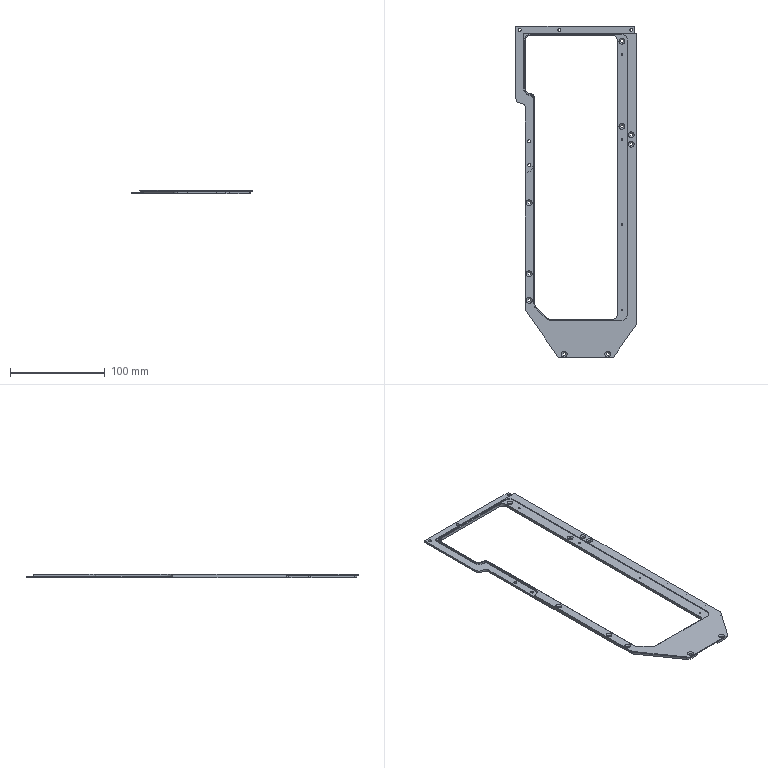NC program | NX | posted with a generic post | part box 127 x 351 x 4 mm
Whole program:
N10 G17 G21 G94 G90
(DRILL_HOLES , TOOL : CHAMFER_D8-90DEG)
N12 T01 M6
N14 G53
N16 G17 G0 G90 X153.952 Y-40.61 S2500 M3
N18 G43 Z20. H1
N20 G94 G82 G98 Z-2.6 F250. P200 R3.
N22 X103.952 Y-30.61
N24 X48.952
N26 X-6.048
N28 X-61.048
N30 X-111.048
N32 X-101. Y3.5
N34 X-111.048 Y28.911
N36 X-61.048
N38 X-6.048
N40 X48.952
N42 X103.952
N44 X119. Y3.5
N46 X153.952 Y28.911
N48 G80
N50 G0 X153.952 Y28.911 Z20.
(DRILL_HOLES_1_COPY_1 , TOOL : CHAMFER_D8-90DEG)
N52 X-168. Y33.5
N54 G82 Z-1.6 F250. P200 R3.
N56 Y-12.5
N58 G80
N60 G0 X-168. Y-12.5 Z20.
N62 M5
(DRILL_HOLES_COPY , TOOL : DRILL_D5.3-62-92)
N64 T02 M6
N66 G53
N68 G17 G0 G90 X153.952 Y-40.61 S3000 M3
N70 G43 Z20. H2
N72 G94 G82 G98 Z-6.5 F200. P200 R3.
N74 X103.952 Y-30.61
N76 X48.952
N78 X-6.048
N80 X-61.048
N82 X-111.048
N84 X-101. Y3.5
N86 X-111.048 Y28.911
N88 X-61.048
N90 X-6.048
N92 X48.952
N94 X103.952
N96 X119. Y3.5
N98 X153.952 Y28.911
N100 G80
N102 G0 X153.952 Y28.911 Z20.
N104 M5
(DRILL_HOLES_1_COPY_COPY , TOOL : DRILL_D3.2-42-71)
N106 T06 M6
N108 G53
N110 G17 G0 G90 X-168. Y33.5 S3000 M3
N112 G43 Z20. H6
N114 G94 G82 G98 Z-6. F200. P200 R3.
N116 Y-12.5
N118 G80
N120 G0 X-168. Y-12.5 Z20.
N122 M5
(PLANAR_MILL_7_COPY_1_COPY , TOOL : CHAMFER_D3-90DEG)
N124 T08 M6
N126 G53
N128 G17 G0 G90 X-167.152 Y-21.454 S3000 M3
N130 G43 Z20. H8
N132 Z2.
N134 G94 G1 Z-1. F300.
N136 G41 X-167.294 Y-21.313 D8
N138 X-168.113 Y-20.739
N140 X-169.341 Y-19.879
N142 G2 X-171.9 Y-14.964 R6.
N144 G1 Y-4.5
N146 G2 X-170.9 Y-3.5 R1.
N148 G1 X-162.
N150 G2 X-161. Y-4.5 R1.
N152 G1 Y-10.5
N154 G3 X-157. Y-14.5 R4.
N156 G1 X-131.
N158 X-128.5
N160 G40
N162 X-128.303 Y-14.465
N164 Z2.
N166 G0 Z20.
N168 Y35.465
N170 Z2.
N172 G1 Z-1.
N174 G41 X-128.5 Y35.5
N176 X-129.5
N178 X-131.
N180 X-157.
N182 G3 X-161. Y31.5 R4.
N184 G1 Y25.5
N186 G2 X-162. Y24.5 R1.
N188 G1 X-170.9
N190 G2 X-171.9 Y25.5 R1.
N192 G1 Y35.817
N194 G2 X-169.341 Y40.732 R6.
N196 G1 X-167.294 Y42.166
N198 G40
N200 X-167.152 Y42.308
N202 Z2.
N204 G0 Z20.
(PLANAR_MILL_7_COPY_1_COPY_COPY , TOOL : CHAMFER_D3-90DEG)
N206 Y-21.454
N208 Z2.
N210 G1 Z-1.
N212 G41 X-167.294 Y-21.313
N214 X-168.113 Y-20.739
N216 X-169.341 Y-19.879
N218 G2 X-171.9 Y-14.964 R6.
N220 G1 Y-4.5
N222 G2 X-170.9 Y-3.5 R1.
N224 G1 X-162.
N226 G2 X-161. Y-4.5 R1.
N228 G1 Y-10.5
N230 G3 X-157. Y-14.5 R4.
N232 G1 X-131.
N234 X-128.5
N236 G40
N238 X-128.303 Y-14.465
N240 Z2.
N242 G0 Z20.
N244 Y35.465
N246 Z2.
N248 G1 Z-1.
N250 G41 X-128.5 Y35.5
N252 X-129.5
N254 X-131.
N256 X-157.
N258 G3 X-161. Y31.5 R4.
N260 G1 Y25.5
N262 G2 X-162. Y24.5 R1.
N264 G1 X-170.9
N266 G2 X-171.9 Y25.5 R1.
N268 G1 Y35.817
N270 G2 X-169.341 Y40.732 R6.
N272 G1 X-167.294 Y42.166
N274 G40
N276 X-167.152 Y42.308
N278 Z2.
N280 G0 Z20.
N282 M5
(DRILL_HOLES_1 , TOOL : CHAMFER_D8-90DEG)
N284 T01 M6
N286 G53
N288 G17 G0 G90 X-111. Y-49.5 S2500 M3
N290 G43 Z20. H1
N292 G94 G82 G98 Z-1.6 F250. P200 R3.
N294 X-83.
N296 X-8.
N298 X32.
N300 X57.
N302 X175. Y-59.5
N304 Y-17.5
N306 Y58.5
N308 X163. Y48.5
N310 X73.
N312 X64. Y58.5
N314 X54.
N316 G80
N318 G0 X54. Y58.5 Z20.
N320 M5
(DRILL_HOLES_1_COPY , TOOL : DRILL_D3.2-42-71)
N322 T06 M6
N324 G53
N326 G17 G0 G90 X-111. Y-49.5 S3000 M3
N328 G43 Z20. H6
N330 G94 G82 G98 Z-6. F200. P200 R3.
N332 X-83.
N334 X-8.
N336 X32.
N338 X57.
N340 X175. Y-59.5
N342 Y-17.5
N344 Y58.5
N346 X163. Y48.5
N348 X73.
N350 X64. Y58.5
N352 X54.
N354 G80
N356 G0 X54. Y58.5 Z20.
N358 M5
(PLANAR_MILL_8 , TOOL : D6-18-D6-50-3T-ROUGH)
N360 T03 M6
N362 G53
N364 G17 G0 G90 X-99.181 Y2.877 S3500 M3
N366 G43 Z20. H3
N368 Z1.
N370 G94 G1 X-99.078 Y3.67 Z0.979 F1500.
N372 X-99.329 Y4.465 Z0.957
N374 X-99.891 Y5.08 Z0.935
N376 X-100.661 Y5.4 Z0.914
N378 X-101.339 Z0.896
N380 X-102.109 Y5.08 Z0.874
N382 X-102.671 Y4.465 Z0.852
N384 X-102.922 Y3.67 Z0.83
N386 X-102.815 Y2.844 Z0.809
N388 X-102.476 Y2.256 Z0.791
N390 X-101.965 Y1.829 Z0.773
N392 X-101.339 Y1.6 Z0.756
N394 X-100.661 Z0.738
N396 X-100.035 Y1.829 Z0.721
N398 X-99.524 Y2.256 Z0.703
N400 X-99.185 Y2.844 Z0.685
N402 X-99.078 Y3.67 Z0.664
N404 X-99.329 Y4.465 Z0.642
N406 X-99.891 Y5.08 Z0.62
N408 X-100.661 Y5.4 Z0.598
N410 X-101.339 Z0.58
N412 X-102.109 Y5.08 Z0.559
N414 X-102.671 Y4.465 Z0.537
N416 X-102.922 Y3.67 Z0.515
N418 X-102.815 Y2.844 Z0.493
N420 X-102.476 Y2.256 Z0.475
N422 X-101.965 Y1.829 Z0.458
N424 X-101.339 Y1.6 Z0.44
N426 X-100.661 Z0.423
N428 X-100.035 Y1.829 Z0.405
N430 X-99.524 Y2.256 Z0.388
N432 X-99.185 Y2.844 Z0.37
N434 X-99.078 Y3.67 Z0.348
N436 X-99.329 Y4.465 Z0.326
N438 X-99.891 Y5.08 Z0.305
N440 X-100.661 Y5.4 Z0.283
N442 X-101.339 Z0.265
N444 X-102.109 Y5.08 Z0.243
N446 X-102.671 Y4.465 Z0.221
N448 X-102.922 Y3.67 Z0.199
N450 X-102.815 Y2.844 Z0.178
N452 X-102.476 Y2.256 Z0.16
N454 X-101.965 Y1.829 Z0.142
N456 X-101.339 Y1.6 Z0.125
N458 X-100.661 Z0.107
N460 X-100.035 Y1.829 Z0.09
N462 X-99.524 Y2.256 Z0.072
N464 X-99.185 Y2.844 Z0.055
N466 X-99.078 Y3.67 Z0.033
N468 X-99.329 Y4.465 Z0.011
N470 X-99.891 Y5.08 Z-0.011
N472 X-100.661 Y5.4 Z-0.033
N474 X-101.339 Z-0.05
N476 X-102.109 Y5.08 Z-0.072
N478 X-102.671 Y4.465 Z-0.094
N480 X-102.922 Y3.67 Z-0.116
N482 X-102.815 Y2.844 Z-0.138
N484 X-102.476 Y2.256 Z-0.156
N486 X-101.965 Y1.829 Z-0.173
N488 X-101.339 Y1.6 Z-0.19
N490 X-100.661 Z-0.208
N492 X-100.035 Y1.829 Z-0.226
N494 X-99.524 Y2.256 Z-0.243
N496 X-99.185 Y2.844 Z-0.261
N498 X-99.078 Y3.67 Z-0.283
N500 X-99.329 Y4.465 Z-0.305
N502 X-99.891 Y5.08 Z-0.326
N504 X-100.661 Y5.4 Z-0.348
N506 X-101.339 Z-0.366
N508 X-102.109 Y5.08 Z-0.388
N510 X-102.671 Y4.465 Z-0.41
N512 X-102.922 Y3.67 Z-0.431
N514 X-102.815 Y2.844 Z-0.453
N516 X-102.476 Y2.256 Z-0.471
N518 X-101.965 Y1.829 Z-0.488
N520 X-101.339 Y1.6 Z-0.506
N522 X-100.661 Z-0.524
N524 X-100.035 Y1.829 Z-0.541
N526 X-99.524 Y2.256 Z-0.559
N528 X-99.185 Y2.844 Z-0.576
N530 X-99.078 Y3.67 Z-0.598
N532 X-99.329 Y4.465 Z-0.62
N534 X-99.891 Y5.08 Z-0.642
N536 X-100.661 Y5.4 Z-0.664
N538 X-101.339 Z-0.681
N540 X-102.109 Y5.08 Z-0.703
N542 X-102.671 Y4.465 Z-0.725
N544 X-102.922 Y3.67 Z-0.747
N546 X-102.815 Y2.844 Z-0.769
N548 X-102.476 Y2.256 Z-0.786
N550 X-101.965 Y1.829 Z-0.804
N552 X-101.339 Y1.6 Z-0.821
N554 X-100.661 Z-0.839
N556 X-100.035 Y1.829 Z-0.857
N558 X-99.524 Y2.256 Z-0.874
N560 X-99.185 Y2.844 Z-0.892
N562 X-99.078 Y3.67 Z-0.914
N564 X-99.329 Y4.465 Z-0.935
N566 X-99.891 Y5.08 Z-0.957
N568 X-100.661 Y5.4 Z-0.979
N570 X-101.339 Z-0.997
N572 X-102.109 Y5.08 Z-1.019
N574 X-102.671 Y4.465 Z-1.04
N576 X-102.922 Y3.67 Z-1.062
N578 X-102.815 Y2.844 Z-1.084
N580 X-102.476 Y2.256 Z-1.102
N582 X-101.965 Y1.829 Z-1.119
N584 X-101.339 Y1.6 Z-1.137
N586 X-100.661 Z-1.155
N588 X-100.035 Y1.829 Z-1.172
N590 X-99.524 Y2.256 Z-1.189
N592 X-99.185 Y2.844 Z-1.207
N594 X-99.078 Y3.67 Z-1.229
N596 X-99.329 Y4.465 Z-1.251
N598 X-99.891 Y5.08 Z-1.273
N600 X-100.661 Y5.4 Z-1.294
N602 X-101.339 Z-1.312
N604 X-102.109 Y5.08 Z-1.334
N606 X-102.671 Y4.465 Z-1.356
N608 X-102.922 Y3.67 Z-1.378
N610 X-102.815 Y2.844 Z-1.4
N612 X-102.476 Y2.256 Z-1.417
N614 X-101.965 Y1.829 Z-1.435
N616 X-101.339 Y1.6 Z-1.452
N618 X-100.661 Z-1.47
N620 X-100.035 Y1.829 Z-1.487
N622 X-99.524 Y2.256 Z-1.505
N624 X-99.185 Y2.844 Z-1.523
N626 X-99.078 Y3.67 Z-1.544
N628 X-99.329 Y4.465 Z-1.566
N630 X-99.891 Y5.08 Z-1.588
N632 X-100.661 Y5.4 Z-1.61
N634 X-101.339 Z-1.628
N636 X-102.109 Y5.08 Z-1.649
N638 X-102.671 Y4.465 Z-1.671
N640 X-102.922 Y3.67 Z-1.693
N642 X-102.815 Y2.844 Z-1.715
N644 X-102.476 Y2.256 Z-1.733
N646 X-101.965 Y1.829 Z-1.75
N648 X-101.339 Y1.6 Z-1.768
N650 X-100.661 Z-1.785
N652 X-100.035 Y1.829 Z-1.803
N654 X-99.524 Y2.256 Z-1.82
N656 X-99.185 Y2.844 Z-1.838
N658 X-99.078 Y3.67 Z-1.86
N660 X-99.329 Y4.465 Z-1.882
N662 X-99.891 Y5.08 Z-1.904
N664 X-100.661 Y5.4 Z-1.925
N666 X-101.339 Z-1.943
N668 X-102.109 Y5.08 Z-1.965
N670 X-102.671 Y4.465 Z-1.987
N672 X-102.922 Y3.67 Z-2.009
N674 X-102.815 Y2.844 Z-2.03
N676 X-102.476 Y2.256 Z-2.048
N678 X-101.965 Y1.829 Z-2.066
N680 X-101.339 Y1.6 Z-2.083
N682 X-100.661 Z-2.101
N684 X-100.035 Y1.829 Z-2.118
N686 X-99.524 Y2.256 Z-2.136
N688 X-99.185 Y2.844 Z-2.153
N690 X-99.078 Y3.67 Z-2.175
N692 X-99.329 Y4.465 Z-2.197
N694 X-99.891 Y5.08 Z-2.219
N696 X-100.661 Y5.4 Z-2.241
N698 X-101.339 Z-2.259
N700 X-102.109 Y5.08 Z-2.28
N702 X-102.671 Y4.465 Z-2.302
N704 X-102.922 Y3.67 Z-2.324
N706 X-102.815 Y2.844 Z-2.346
N708 X-102.476 Y2.256 Z-2.364
N710 X-101.965 Y1.829 Z-2.381
N712 X-101.339 Y1.6 Z-2.399
N714 X-100.661 Z-2.416
N716 X-100.035 Y1.829 Z-2.434
N718 X-99.524 Y2.256 Z-2.451
N720 X-99.185 Y2.844 Z-2.469
N722 X-99.078 Y3.67 Z-2.491
N724 X-99.329 Y4.465 Z-2.513
N726 X-99.891 Y5.08 Z-2.534
N728 X-100.661 Y5.4 Z-2.556
N730 X-101.339 Z-2.574
N732 X-102.109 Y5.08 Z-2.596
N734 X-102.671 Y4.465 Z-2.618
N736 X-102.922 Y3.67 Z-2.639
N738 X-102.815 Y2.844 Z-2.661
N740 X-102.476 Y2.256 Z-2.679
N742 X-101.965 Y1.829 Z-2.696
N744 X-101.339 Y1.6 Z-2.714
N746 X-100.661 Z-2.732
N748 X-100.035 Y1.829 Z-2.749
N750 X-99.524 Y2.256 Z-2.767
N752 X-99.185 Y2.844 Z-2.784
N754 X-99.078 Y3.67 Z-2.806
N756 X-99.329 Y4.465 Z-2.828
N758 X-99.891 Y5.08 Z-2.85
N760 X-100.661 Y5.4 Z-2.872
N762 X-101.339 Z-2.889
N764 X-102.109 Y5.08 Z-2.911
N766 X-102.671 Y4.465 Z-2.933
N768 X-102.922 Y3.67 Z-2.955
N770 X-102.815 Y2.844 Z-2.977
N772 X-102.476 Y2.256 Z-2.994
N774 X-101.965 Y1.829 Z-3.012
N776 X-101.339 Y1.6 Z-3.029
N778 X-100.661 Z-3.047
N780 X-100.035 Y1.829 Z-3.065
N782 X-99.524 Y2.256 Z-3.082
N784 X-99.185 Y2.844 Z-3.1
N786 X-99.078 Y3.67 Z-3.122
N788 X-99.329 Y4.465 Z-3.143
N790 X-99.891 Y5.08 Z-3.165
N792 X-100.661 Y5.4 Z-3.187
N794 X-101.339 Z-3.205
N796 X-102.109 Y5.08 Z-3.227
N798 X-102.671 Y4.465 Z-3.249
N800 X-102.922 Y3.67 Z-3.27
N802 X-102.815 Y2.844 Z-3.292
N804 X-102.476 Y2.256 Z-3.31
N806 X-101.965 Y1.829 Z-3.327
N808 X-101.339 Y1.6 Z-3.345
N810 X-100.661 Z-3.363
N812 X-100.035 Y1.829 Z-3.38
N814 X-99.524 Y2.256 Z-3.397
N816 X-99.185 Y2.844 Z-3.415
N818 X-99.078 Y3.67 Z-3.437
N820 X-99.329 Y4.465 Z-3.459
N822 X-99.891 Y5.08 Z-3.481
N824 X-100.661 Y5.4 Z-3.503
N826 X-101.339 Z-3.52
N828 X-102.109 Y5.08 Z-3.542
N830 X-102.671 Y4.465 Z-3.564
N832 X-102.922 Y3.67 Z-3.586
N834 X-102.815 Y2.844 Z-3.608
N836 X-102.476 Y2.256 Z-3.625
N838 X-101.965 Y1.829 Z-3.643
N840 X-101.339 Y1.6 Z-3.66
N842 X-100.661 Z-3.678
N844 X-100.035 Y1.829 Z-3.695
N846 X-99.524 Y2.256 Z-3.713
N848 X-99.185 Y2.844 Z-3.731
N850 X-99.078 Y3.67 Z-3.752
N852 X-99.329 Y4.465 Z-3.774
N854 X-99.891 Y5.08 Z-3.796
N856 X-100.661 Y5.4 Z-3.818
N858 X-101.339 Z-3.836
N860 X-102.109 Y5.08 Z-3.858
N862 X-102.671 Y4.465 Z-3.879
N864 X-102.922 Y3.67 Z-3.901
N866 X-102.815 Y2.844 Z-3.923
N868 X-102.476 Y2.256 Z-3.941
N870 X-101.965 Y1.829 Z-3.958
N872 X-101.339 Y1.6 Z-3.976
N874 X-100.661 Z-3.993
N876 X-100.035 Y1.829 Z-4.011
N878 X-99.524 Y2.256 Z-4.028
N880 X-99.185 Y2.844 Z-4.046
N882 X-99.078 Y3.67 Z-4.068
N884 X-99.329 Y4.465 Z-4.09
N886 X-99.891 Y5.08 Z-4.112
N888 X-100.661 Y5.4 Z-4.133
N890 X-101.339 Z-4.151
N892 X-102.109 Y5.08 Z-4.173
N894 X-102.671 Y4.465 Z-4.195
N896 X-102.922 Y3.67 Z-4.217
N898 X-102.815 Y2.844 Z-4.238
N900 X-102.476 Y2.256 Z-4.256
N902 X-101.965 Y1.829 Z-4.274
N904 X-101.339 Y1.6 Z-4.291
N906 X-101. Z-4.3
N908 G3 X-99.1 Y3.5 R1.9
N910 X-101. Y1.6 R-1.9
N912 G1 Z-3.3
N914 G0 Z20.
N916 X120.819 Y2.877
N918 Z1.
N920 G1 X120.922 Y3.67 Z0.979
N922 X120.671 Y4.465 Z0.957
N924 X120.109 Y5.08 Z0.935
N926 X119.339 Y5.4 Z0.914
N928 X118.661 Z0.896
N930 X117.891 Y5.08 Z0.874
N932 X117.329 Y4.465 Z0.852
N934 X117.078 Y3.67 Z0.83
N936 X117.185 Y2.844 Z0.809
N938 X117.524 Y2.256 Z0.791
N940 X118.035 Y1.829 Z0.773
N942 X118.661 Y1.6 Z0.756
N944 X119.339 Z0.738
N946 X119.965 Y1.829 Z0.721
N948 X120.476 Y2.256 Z0.703
N950 X120.815 Y2.844 Z0.685
N952 X120.922 Y3.67 Z0.664
N954 X120.671 Y4.465 Z0.642
N956 X120.109 Y5.08 Z0.62
N958 X119.339 Y5.4 Z0.598
N960 X118.661 Z0.58
N962 X117.891 Y5.08 Z0.559
N964 X117.329 Y4.465 Z0.537
N966 X117.078 Y3.67 Z0.515
N968 X117.185 Y2.844 Z0.493
N970 X117.524 Y2.256 Z0.475
N972 X118.035 Y1.829 Z0.458
N974 X118.661 Y1.6 Z0.44
N976 X119.339 Z0.423
N978 X119.965 Y1.829 Z0.405
N980 X120.476 Y2.256 Z0.388
N982 X120.815 Y2.844 Z0.37
N984 X120.922 Y3.67 Z0.348
N986 X120.671 Y4.465 Z0.326
N988 X120.109 Y5.08 Z0.305
N990 X119.339 Y5.4 Z0.283
N992 X118.661 Z0.265
N994 X117.891 Y5.08 Z0.243
N996 X117.329 Y4.465 Z0.221
N998 X117.078 Y3.67 Z0.199
N1000 X117.185 Y2.844 Z0.178
N1002 X117.524 Y2.256 Z0.16
N1004 X118.035 Y1.829 Z0.142
N1006 X118.661 Y1.6 Z0.125
N1008 X119.339 Z0.107
N1010 X119.965 Y1.829 Z0.09
N1012 X120.476 Y2.256 Z0.072
N1014 X120.815 Y2.844 Z0.055
N1016 X120.922 Y3.67 Z0.033
N1018 X120.671 Y4.465 Z0.011
N1020 X120.109 Y5.08 Z-0.011
N1022 X119.339 Y5.4 Z-0.033
N1024 X118.661 Z-0.05
N1026 X117.891 Y5.08 Z-0.072
N1028 X117.329 Y4.465 Z-0.094
N1030 X117.078 Y3.67 Z-0.116
N1032 X117.185 Y2.844 Z-0.138
N1034 X117.524 Y2.256 Z-0.156
N1036 X118.035 Y1.829 Z-0.173
N1038 X118.661 Y1.6 Z-0.19
N1040 X119.339 Z-0.208
N1042 X119.965 Y1.829 Z-0.226
N1044 X120.476 Y2.256 Z-0.243
N1046 X120.815 Y2.844 Z-0.261
N1048 X120.922 Y3.67 Z-0.283
N1050 X120.671 Y4.465 Z-0.305
N1052 X120.109 Y5.08 Z-0.326
N1054 X119.339 Y5.4 Z-0.348
N1056 X118.661 Z-0.366
N1058 X117.891 Y5.08 Z-0.388
N1060 X117.329 Y4.465 Z-0.41
N1062 X117.078 Y3.67 Z-0.431
N1064 X117.185 Y2.844 Z-0.453
N1066 X117.524 Y2.256 Z-0.471
N1068 X118.035 Y1.829 Z-0.488
N1070 X118.661 Y1.6 Z-0.506
N1072 X119.339 Z-0.524
N1074 X119.965 Y1.829 Z-0.541
N1076 X120.476 Y2.256 Z-0.559
N1078 X120.815 Y2.844 Z-0.576
N1080 X120.922 Y3.67 Z-0.598
N1082 X120.671 Y4.465 Z-0.62
N1084 X120.109 Y5.08 Z-0.642
N1086 X119.339 Y5.4 Z-0.664
N1088 X118.661 Z-0.681
N1090 X117.891 Y5.08 Z-0.703
N1092 X117.329 Y4.465 Z-0.725
N1094 X117.078 Y3.67 Z-0.747
N1096 X117.185 Y2.844 Z-0.769
N1098 X117.524 Y2.256 Z-0.786
N1100 X118.035 Y1.829 Z-0.804
N1102 X118.661 Y1.6 Z-0.821
N1104 X119.339 Z-0.839
N1106 X119.965 Y1.829 Z-0.857
N1108 X120.476 Y2.256 Z-0.874
N1110 X120.815 Y2.844 Z-0.892
N1112 X120.922 Y3.67 Z-0.914
N1114 X120.671 Y4.465 Z-0.935
N1116 X120.109 Y5.08 Z-0.957
N1118 X119.339 Y5.4 Z-0.979
N1120 X118.661 Z-0.997
N1122 X117.891 Y5.08 Z-1.019
N1124 X117.329 Y4.465 Z-1.04
N1126 X117.078 Y3.67 Z-1.062
N1128 X117.185 Y2.844 Z-1.084
N1130 X117.524 Y2.256 Z-1.102
N1132 X118.035 Y1.829 Z-1.119
N1134 X118.661 Y1.6 Z-1.137
N1136 X119.339 Z-1.155
N1138 X119.965 Y1.829 Z-1.172
N1140 X120.476 Y2.256 Z-1.189
N1142 X120.815 Y2.844 Z-1.207
N1144 X120.922 Y3.67 Z-1.229
N1146 X120.671 Y4.465 Z-1.251
N1148 X120.109 Y5.08 Z-1.273
N1150 X119.339 Y5.4 Z-1.294
N1152 X118.661 Z-1.312
N1154 X117.891 Y5.08 Z-1.334
N1156 X117.329 Y4.465 Z-1.356
N1158 X117.078 Y3.67 Z-1.378
N1160 X117.185 Y2.844 Z-1.4
N1162 X117.524 Y2.256 Z-1.417
N1164 X118.035 Y1.829 Z-1.435
N1166 X118.661 Y1.6 Z-1.452
N1168 X119.339 Z-1.47
N1170 X119.965 Y1.829 Z-1.487
N1172 X120.476 Y2.256 Z-1.505
N1174 X120.815 Y2.844 Z-1.523
N1176 X120.922 Y3.67 Z-1.544
N1178 X120.671 Y4.465 Z-1.566
N1180 X120.109 Y5.08 Z-1.588
N1182 X119.339 Y5.4 Z-1.61
N1184 X118.661 Z-1.628
N1186 X117.891 Y5.08 Z-1.649
N1188 X117.329 Y4.465 Z-1.671
N1190 X117.078 Y3.67 Z-1.693
N1192 X117.185 Y2.844 Z-1.715
N1194 X117.524 Y2.256 Z-1.733
N1196 X118.035 Y1.829 Z-1.75
N1198 X118.661 Y1.6 Z-1.768
N1200 X119.339 Z-1.785
N1202 X119.965 Y1.829 Z-1.803
N1204 X120.476 Y2.256 Z-1.82
N1206 X120.815 Y2.844 Z-1.838
N1208 X120.922 Y3.67 Z-1.86
N1210 X120.671 Y4.465 Z-1.882
N1212 X120.109 Y5.08 Z-1.904
N1214 X119.339 Y5.4 Z-1.925
N1216 X118.661 Z-1.943
N1218 X117.891 Y5.08 Z-1.965
N1220 X117.329 Y4.465 Z-1.987
N1222 X117.078 Y3.67 Z-2.009
N1224 X117.185 Y2.844 Z-2.03
N1226 X117.524 Y2.256 Z-2.048
N1228 X118.035 Y1.829 Z-2.066
N1230 X118.661 Y1.6 Z-2.083
N1232 X119.339 Z-2.101
N1234 X119.965 Y1.829 Z-2.118
N1236 X120.476 Y2.256 Z-2.136
N1238 X120.815 Y2.844 Z-2.153
N1240 X120.922 Y3.67 Z-2.175
N1242 X120.671 Y4.465 Z-2.197
N1244 X120.109 Y5.08 Z-2.219
N1246 X119.339 Y5.4 Z-2.241
N1248 X118.661 Z-2.259
N1250 X117.891 Y5.08 Z-2.28
N1252 X117.329 Y4.465 Z-2.302
N1254 X117.078 Y3.67 Z-2.324
N1256 X117.185 Y2.844 Z-2.346
N1258 X117.524 Y2.256 Z-2.364
N1260 X118.035 Y1.829 Z-2.381
N1262 X118.661 Y1.6 Z-2.399
N1264 X119.339 Z-2.416
N1266 X119.965 Y1.829 Z-2.434
N1268 X120.476 Y2.256 Z-2.451
N1270 X120.815 Y2.844 Z-2.469
N1272 X120.922 Y3.67 Z-2.491
N1274 X120.671 Y4.465 Z-2.513
N1276 X120.109 Y5.08 Z-2.534
N1278 X119.339 Y5.4 Z-2.556
N1280 X118.661 Z-2.574
N1282 X117.891 Y5.08 Z-2.596
N1284 X117.329 Y4.465 Z-2.618
N1286 X117.078 Y3.67 Z-2.639
N1288 X117.185 Y2.844 Z-2.661
N1290 X117.524 Y2.256 Z-2.679
N1292 X118.035 Y1.829 Z-2.696
N1294 X118.661 Y1.6 Z-2.714
N1296 X119.339 Z-2.732
N1298 X119.965 Y1.829 Z-2.749
N1300 X120.476 Y2.256 Z-2.767
N1302 X120.815 Y2.844 Z-2.784
N1304 X120.922 Y3.67 Z-2.806
N1306 X120.671 Y4.465 Z-2.828
N1308 X120.109 Y5.08 Z-2.85
N1310 X119.339 Y5.4 Z-2.872
N1312 X118.661 Z-2.889
N1314 X117.891 Y5.08 Z-2.911
N1316 X117.329 Y4.465 Z-2.933
N1318 X117.078 Y3.67 Z-2.955
N1320 X117.185 Y2.844 Z-2.977
N1322 X117.524 Y2.256 Z-2.994
N1324 X118.035 Y1.829 Z-3.012
N1326 X118.661 Y1.6 Z-3.029
N1328 X119.339 Z-3.047
N1330 X119.965 Y1.829 Z-3.065
N1332 X120.476 Y2.256 Z-3.082
N1334 X120.815 Y2.844 Z-3.1
N1336 X120.922 Y3.67 Z-3.122
N1338 X120.671 Y4.465 Z-3.143
N1340 X120.109 Y5.08 Z-3.165
N1342 X119.339 Y5.4 Z-3.187
N1344 X118.661 Z-3.205
N1346 X117.891 Y5.08 Z-3.227
N1348 X117.329 Y4.465 Z-3.249
N1350 X117.078 Y3.67 Z-3.27
N1352 X117.185 Y2.844 Z-3.292
N1354 X117.524 Y2.256 Z-3.31
N1356 X118.035 Y1.829 Z-3.327
N1358 X118.661 Y1.6 Z-3.345
N1360 X119.339 Z-3.363
N1362 X119.965 Y1.829 Z-3.38
N1364 X120.476 Y2.256 Z-3.397
N1366 X120.815 Y2.844 Z-3.415
N1368 X120.922 Y3.67 Z-3.437
N1370 X120.671 Y4.465 Z-3.459
N1372 X120.109 Y5.08 Z-3.481
N1374 X119.339 Y5.4 Z-3.503
N1376 X118.661 Z-3.52
N1378 X117.891 Y5.08 Z-3.542
N1380 X117.329 Y4.465 Z-3.564
N1382 X117.078 Y3.67 Z-3.586
N1384 X117.185 Y2.844 Z-3.608
N1386 X117.524 Y2.256 Z-3.625
N1388 X118.035 Y1.829 Z-3.643
N1390 X118.661 Y1.6 Z-3.66
N1392 X119.339 Z-3.678
N1394 X119.965 Y1.829 Z-3.695
N1396 X120.476 Y2.256 Z-3.713
N1398 X120.815 Y2.844 Z-3.731
N1400 X120.922 Y3.67 Z-3.752
N1402 X120.671 Y4.465 Z-3.774
N1404 X120.109 Y5.08 Z-3.796
N1406 X119.339 Y5.4 Z-3.818
N1408 X118.661 Z-3.836
N1410 X117.891 Y5.08 Z-3.858
N1412 X117.329 Y4.465 Z-3.879
N1414 X117.078 Y3.67 Z-3.901
N1416 X117.185 Y2.844 Z-3.923
N1418 X117.524 Y2.256 Z-3.941
N1420 X118.035 Y1.829 Z-3.958
N1422 X118.661 Y1.6 Z-3.976
N1424 X119.339 Z-3.993
N1426 X119.965 Y1.829 Z-4.011
N1428 X120.476 Y2.256 Z-4.028
N1430 X120.815 Y2.844 Z-4.046
N1432 X120.922 Y3.67 Z-4.068
N1434 X120.671 Y4.465 Z-4.09
N1436 X120.109 Y5.08 Z-4.112
N1438 X119.339 Y5.4 Z-4.133
N1440 X118.661 Z-4.151
N1442 X117.891 Y5.08 Z-4.173
N1444 X117.329 Y4.465 Z-4.195
N1446 X117.078 Y3.67 Z-4.217
N1448 X117.185 Y2.844 Z-4.238
N1450 X117.524 Y2.256 Z-4.256
N1452 X118.035 Y1.829 Z-4.274
N1454 X118.661 Y1.6 Z-4.291
N1456 X119. Z-4.3
N1458 G3 X120.9 Y3.5 R1.9
N1460 X119. Y1.6 R-1.9
N1462 G1 Z-3.3
N1464 G0 Z20.
(FLOOR_FACING , TOOL : D6-18-D6-50-3T-ROUGH)
N1466 X-176.9 Y8.741
N1468 Z2.2
N1470 G1 Z-0.8
N1472 X-170.9
N1474 G3 X-169.4 Y10.241 R1.5
N1476 G1 Y22.4
N1478 X-158.9
N1480 Y31.5
N1482 G2 X-157. Y33.4 R1.9
N1484 G1 X-132.5
N1486 Y-12.4
N1488 X-157.
N1490 G2 X-158.9 Y-10.5 R1.9
N1492 G1 Y-1.4
N1494 X-169.4
N1496 Y10.241
N1498 X-164.9
N1500 Y17.9
N1502 X-158.9
N1504 G3 X-154.4 Y22.4 R4.5
N1506 G1 Y28.9
N1508 X-137.
N1510 Y-7.9
N1512 X-154.4
N1514 Y-1.4
N1516 G3 X-158.9 Y3.1 R4.5
N1518 G1 X-164.9
N1520 Y10.241
N1522 X-160.4
N1524 Y13.4
N1526 X-158.9
N1528 G3 X-149.9 Y22.4 R9.
N1530 G1 Y24.4
N1532 X-141.5
N1534 Y-3.4
N1536 X-149.9
N1538 Y-1.4
N1540 G3 X-158.9 Y7.6 R9.
N1542 G1 X-160.4
N1544 Y10.241
N1546 X-152.525 Y10.5
N1548 G3 X-146. Y18.42 R13.5
N1550 G1 X-144.83 Y21.285
N1552 X-146. Y18.42
N1554 X-146.766 Y21.358
N1556 X-146. Y18.42
N1558 Y2.58
N1560 X-144.83 Y-0.285
N1562 X-146. Y2.58
N1564 X-146.766 Y-0.358
N1566 X-146. Y2.58
N1568 G3 X-152.525 Y10.5 R13.5
N1570 X-151.662 Y11.004 R13.5
N1572 X-151.2 Y13.075 R1.5
N1574 G1 Z2.2
N1576 G0 Z20.
N1578 X-176.9 Y8.741
N1580 Z1.4
N1582 G1 Z-1.6
N1584 X-170.9
N1586 G3 X-169.4 Y10.241 R1.5
N1588 G1 Y22.4
N1590 X-158.9
N1592 Y31.5
N1594 G2 X-157. Y33.4 R1.9
N1596 G1 X-132.5
N1598 Y-12.4
N1600 X-157.
N1602 G2 X-158.9 Y-10.5 R1.9
N1604 G1 Y-1.4
N1606 X-169.4
N1608 Y10.241
N1610 X-164.9
N1612 Y17.9
N1614 X-158.9
N1616 G3 X-154.4 Y22.4 R4.5
N1618 G1 Y28.9
N1620 X-137.
N1622 Y-7.9
N1624 X-154.4
N1626 Y-1.4
N1628 G3 X-158.9 Y3.1 R4.5
N1630 G1 X-164.9
N1632 Y10.241
N1634 X-160.4
N1636 Y13.4
N1638 X-158.9
N1640 G3 X-149.9 Y22.4 R9.
N1642 G1 Y24.4
N1644 X-141.5
N1646 Y-3.4
N1648 X-149.9
N1650 Y-1.4
N1652 G3 X-158.9 Y7.6 R9.
N1654 G1 X-160.4
N1656 Y10.241
N1658 X-152.525 Y10.5
N1660 G3 X-146. Y18.42 R13.5
N1662 G1 X-144.83 Y21.285
N1664 X-146. Y18.42
N1666 X-146.766 Y21.358
N1668 X-146. Y18.42
N1670 Y2.58
N1672 X-144.83 Y-0.285
N1674 X-146. Y2.58
N1676 X-146.766 Y-0.358
N1678 X-146. Y2.58
N1680 G3 X-152.525 Y10.5 R13.5
N1682 X-151.662 Y11.004 R13.5
N1684 X-151.2 Y13.075 R1.5
N1686 G1 Z1.4
N1688 G0 Z20.
N1690 X-176.9 Y8.741
N1692 Z0.6
N1694 G1 Z-2.4
N1696 X-170.9
N1698 G3 X-169.4 Y10.241 R1.5
N1700 G1 Y22.4
N1702 X-158.9
N1704 Y31.5
N1706 G2 X-157. Y33.4 R1.9
N1708 G1 X-132.5
N1710 Y-12.4
N1712 X-157.
N1714 G2 X-158.9 Y-10.5 R1.9
N1716 G1 Y-1.4
N1718 X-169.4
N1720 Y10.241
N1722 X-164.9
N1724 Y17.9
N1726 X-158.9
N1728 G3 X-154.4 Y22.4 R4.5
N1730 G1 Y28.9
N1732 X-137.
N1734 Y-7.9
N1736 X-154.4
N1738 Y-1.4
N1740 G3 X-158.9 Y3.1 R4.5
N1742 G1 X-164.9
N1744 Y10.241
N1746 X-160.4
N1748 Y13.4
N1750 X-158.9
N1752 G3 X-149.9 Y22.4 R9.
N1754 G1 Y24.4
N1756 X-141.5
N1758 Y-3.4
N1760 X-149.9
N1762 Y-1.4
N1764 G3 X-158.9 Y7.6 R9.
N1766 G1 X-160.4
N1768 Y10.241
N1770 X-152.525 Y10.5
N1772 G3 X-146. Y18.42 R13.5
N1774 G1 X-144.83 Y21.285
N1776 X-146. Y18.42
N1778 X-146.766 Y21.358
N1780 X-146. Y18.42
N1782 Y2.58
N1784 X-144.83 Y-0.285
N1786 X-146. Y2.58
N1788 X-146.766 Y-0.358
N1790 X-146. Y2.58
N1792 G3 X-152.525 Y10.5 R13.5
N1794 X-151.662 Y11.004 R13.5
N1796 X-151.2 Y13.075 R1.5
N1798 G1 Z0.6
N1800 G0 Z20.
(PLANAR_MILL , TOOL : D6-18-D6-50-3T-ROUGH)
N1802 X-176.9 Y-1.4
N1804 Z0.6
N1806 G1 Z-2.4
N1808 X-170.9
N1810 X-162.
N1812 G2 X-158.9 Y-4.5 R3.1
N1814 G1 Y-10.5
N1816 G3 X-157. Y-12.4 R1.9
N1818 G1 X-134.1
N1820 Y33.4
N1822 X-157.
N1824 G3 X-158.9 Y31.5 R1.9
N1826 G1 Y25.5
N1828 G2 X-162. Y22.4 R3.1
N1830 G1 X-170.9
N1832 X-176.9
N1834 Z0.6
N1836 G0 Z20.
(PLANAR_MILL_1_COPY_1 , TOOL : D6-18-D6-50-3T-ROUGH)
N1838 X185. Y-66.6
N1840 Z2.14
N1842 G1 Z-0.86
N1844 X179.
N1846 X102.5
N1848 G2 X94.4 Y-58.5 R8.1
N1850 G3 X92.5 Y-56.6 R1.9
N1852 G1 X-120.869
N1854 G2 X-123.795 Y-55.678 R5.1
N1856 G1 X-172.925 Y-21.276
N1858 G2 X-175.1 Y-17.098 R5.1
N1860 G1 Y37.952
N1862 G2 X-172.925 Y42.129 R5.1
N1864 G1 X-139.295 Y65.678
N1866 G2 X-136.369 Y66.6 R5.1
N1868 G1 X178.631
N1870 X184.631
N1872 Z2.14
N1874 G0 Z20.
N1876 X185. Y-66.6
N1878 Z1.28
N1880 G1 Z-1.72
N1882 X179.
N1884 X102.5
N1886 G2 X94.4 Y-58.5 R8.1
N1888 G3 X92.5 Y-56.6 R1.9
N1890 G1 X-120.869
N1892 G2 X-123.795 Y-55.678 R5.1
N1894 G1 X-172.925 Y-21.276
N1896 G2 X-175.1 Y-17.098 R5.1
N1898 G1 Y37.952
N1900 G2 X-172.925 Y42.129 R5.1
N1902 G1 X-139.295 Y65.678
N1904 G2 X-136.369 Y66.6 R5.1
N1906 G1 X178.631
N1908 X184.631
N1910 Z1.28
N1912 G0 Z20.
N1914 X185. Y-66.6
N1916 Z0.42
N1918 G1 Z-2.58
N1920 X179.
N1922 X102.5
N1924 G2 X94.4 Y-58.5 R8.1
N1926 G3 X92.5 Y-56.6 R1.9
N1928 G1 X-120.869
N1930 G2 X-123.795 Y-55.678 R5.1
N1932 G1 X-172.925 Y-21.276
N1934 G2 X-175.1 Y-17.098 R5.1
N1936 G1 Y37.952
N1938 G2 X-172.925 Y42.129 R5.1
N1940 G1 X-139.295 Y65.678
N1942 G2 X-136.369 Y66.6 R5.1
N1944 G1 X178.631
N1946 X184.631
N1948 Z0.42
N1950 G0 Z20.
N1952 X185. Y-66.6
N1954 Z-0.44
N1956 G1 Z-3.44
N1958 X179.
N1960 X102.5
N1962 G2 X94.4 Y-58.5 R8.1
N1964 G3 X92.5 Y-56.6 R1.9
N1966 G1 X-120.869
N1968 G2 X-123.795 Y-55.678 R5.1
N1970 G1 X-172.925 Y-21.276
N1972 G2 X-175.1 Y-17.098 R5.1
N1974 G1 Y37.952
N1976 G2 X-172.925 Y42.129 R5.1
N1978 G1 X-139.295 Y65.678
N1980 G2 X-136.369 Y66.6 R5.1
N1982 G1 X178.631
N1984 X184.631
N1986 Z-0.44
N1988 G0 Z20.
N1990 X185. Y-66.6
N1992 Z-1.3
N1994 G1 Z-4.3
N1996 X179.
N1998 X102.5
N2000 G2 X94.4 Y-58.5 R8.1
N2002 G3 X92.5 Y-56.6 R1.9
N2004 G1 X-120.869
N2006 G2 X-123.795 Y-55.678 R5.1
N2008 G1 X-172.925 Y-21.276
N2010 G2 X-175.1 Y-17.098 R5.1
N2012 G1 Y37.952
N2014 G2 X-172.925 Y42.129 R5.1
N2016 G1 X-139.295 Y65.678
N2018 G2 X-136.369 Y66.6 R5.1
N2020 G1 X178.631
N2022 X184.631
N2024 Z-1.3
N2026 G0 Z20.
(PLANAR_MILL_1_COPY_1_COPY , TOOL : D6-18-D6-50-3T-ROUGH)
N2028 X182.1 Y67.5
N2030 Z2.14
N2032 G1 Z-0.86
N2034 Y61.5
N2036 Y-63.5
N2038 Y-69.5
N2040 Z2.14
N2042 G0 Z20.
N2044 Y67.5
N2046 Z1.28
N2048 G1 Z-1.72
N2050 Y61.5
N2052 Y-63.5
N2054 Y-69.5
N2056 Z1.28
N2058 G0 Z20.
N2060 Y67.5
N2062 Z0.42
N2064 G1 Z-2.58
N2066 Y61.5
N2068 Y-63.5
N2070 Y-69.5
N2072 Z0.42
N2074 G0 Z20.
N2076 Y67.5
N2078 Z-0.44
N2080 G1 Z-3.44
N2082 Y61.5
N2084 Y-63.5
N2086 Y-69.5
N2088 Z-0.44
N2090 G0 Z20.
N2092 Y67.5
N2094 Z-1.3
N2096 G1 Z-4.3
N2098 Y61.5
N2100 Y-63.5
N2102 Y-69.5
N2104 Z-1.3
N2106 G0 Z20.
(PLANAR_MILL_1 , TOOL : D6-18-D6-50-3T-ROUGH)
N2108 X-93.06 Y-59.58
N2110 Z2.
N2112 G1 Z-1.
N2114 X-97.86 Y-55.98
N2116 G3 X-99. Y-55.6 R1.9
N2118 G1 X-119.434
N2120 G2 X-124.08 Y-54.135 R8.1
N2122 G1 X-170.546 Y-21.599
N2124 G2 X-174. Y-14.964 R8.1
N2126 G1 Y35.817
N2128 G2 X-170.546 Y42.452 R8.1
N2130 G1 X-141.008 Y63.135
N2132 G2 X-136.362 Y64.6 R8.1
N2134 G1 X170.9
N2136 X176.9
N2138 Z2.
N2140 G0 Z20.
N2142 X-93.06 Y-59.58
N2144 Z1.
N2146 G1 Z-2.
N2148 X-97.86 Y-55.98
N2150 G3 X-99. Y-55.6 R1.9
N2152 G1 X-119.434
N2154 G2 X-124.08 Y-54.135 R8.1
N2156 G1 X-170.546 Y-21.599
N2158 G2 X-174. Y-14.964 R8.1
N2160 G1 Y35.817
N2162 G2 X-170.546 Y42.452 R8.1
N2164 G1 X-141.008 Y63.135
N2166 G2 X-136.362 Y64.6 R8.1
N2168 G1 X170.9
N2170 X176.9
N2172 Z1.
N2174 G0 Z20.
N2176 X-93.06 Y-59.58
N2178 Z0.1
N2180 G1 Z-2.9
N2182 X-97.86 Y-55.98
N2184 G3 X-99. Y-55.6 R1.9
N2186 G1 X-119.434
N2188 G2 X-124.08 Y-54.135 R8.1
N2190 G1 X-170.546 Y-21.599
N2192 G2 X-174. Y-14.964 R8.1
N2194 G1 Y35.817
N2196 G2 X-170.546 Y42.452 R8.1
N2198 G1 X-141.008 Y63.135
N2200 G2 X-136.362 Y64.6 R8.1
N2202 G1 X170.9
N2204 X176.9
N2206 Z0.1
N2208 G0 Z20.
N2210 M5
(PLANAR_MILL_8_COPY , TOOL : D6-18-D6-50-3T-FINISH)
N2212 T04 M6
N2214 G53
N2216 G17 G0 G90 X-101.5 Y2.086 S3500 M3
N2218 G43 Z20. H4
N2220 Z-2.3
N2222 G94 G1 Z-4.3 F300.
N2224 Y2.
N2226 G3 X-101. Y1.5 R0.5
N2228 X-99. Y3.5 R2.
N2230 X-101. Y1.5 R-2.
N2232 X-100.5 Y2. R0.5
N2234 G1 X-101.5
N2236 G3 X-101. Y1.5 R0.5
N2238 X-99. Y3.5 R2.
N2240 X-101. Y1.5 R-2.
N2242 X-100.5 Y2. R0.5
N2244 G1 Y2.086
N2246 Z-2.3
N2248 G0 Z20.
N2250 X118.5
N2252 Z-2.3
N2254 G1 Z-4.3
N2256 Y2.
N2258 G3 X119. Y1.5 R0.5
N2260 X121. Y3.5 R2.
N2262 X119. Y1.5 R-2.
N2264 X119.5 Y2. R0.5
N2266 G1 X118.5
N2268 G3 X119. Y1.5 R0.5
N2270 X121. Y3.5 R2.
N2272 X119. Y1.5 R-2.
N2274 X119.5 Y2. R0.5
N2276 G1 Y2.086
N2278 Z-2.3
N2280 G0 Z20.
(FLOOR_FACING_COPY , TOOL : D6-18-D6-50-3T-FINISH)
N2282 X-176.9 Y8.741
N2284 Z0.5
N2286 G1 Z-2.5 F800.
N2288 X-170.9
N2290 G3 X-169.4 Y10.241 R1.5
N2292 G1 Y22.5
N2294 X-159.
N2296 Y31.5
N2298 G2 X-157. Y33.5 R2.
N2300 G1 X-132.5
N2302 Y-12.5
N2304 X-157.
N2306 G2 X-159. Y-10.5 R2.
N2308 G1 Y-1.5
N2310 X-169.4
N2312 Y10.241
N2314 X-164.9
N2316 Y18.
N2318 X-159.
N2320 G3 X-154.5 Y22.5 R4.5
N2322 G1 Y29.
N2324 X-137.
N2326 Y-8.
N2328 X-154.5
N2330 Y-1.5
N2332 G3 X-159. Y3. R4.5
N2334 G1 X-164.9
N2336 Y10.241
N2338 X-160.4
N2340 Y13.5
N2342 X-159.
N2344 G3 X-150. Y22.5 R9.
N2346 G1 Y24.5
N2348 X-141.5
N2350 Y-3.5
N2352 X-150.
N2354 Y-1.5
N2356 G3 X-159. Y7.5 R9.
N2358 G1 X-160.4
N2360 Y10.241
N2362 X-152.815 Y10.5
N2364 G3 X-146. Y18.86 R13.5
N2366 G1 X-144.525 Y21.486
N2368 X-146. Y18.86
N2370 Y2.14
N2372 X-144.525 Y-0.486
N2374 X-146. Y2.14
N2376 G3 X-152.815 Y10.5 R13.5
N2378 X-151.944 Y10.991 R13.5
N2380 X-151.449 Y13.053 R1.5
N2382 G1 Z0.5
N2384 G0 Z20.
(PLANAR_MILL_COPY , TOOL : D6-18-D6-50-3T-FINISH)
N2386 X-177.097 Y-1.465
N2388 Z0.5
N2390 G1 Z-2.5
N2392 G41 X-176.9 Y-1.5 D4
N2394 X-170.9
N2396 X-162.
N2398 G2 X-159. Y-4.5 R3.
N2400 G1 Y-10.5
N2402 G3 X-157. Y-12.5 R2.
N2404 G1 X-134.
N2406 Y33.5
N2408 X-157.
N2410 G3 X-159. Y31.5 R2.
N2412 G1 Y25.5
N2414 G2 X-162. Y22.5 R3.
N2416 G1 X-170.9
N2418 X-176.9
N2420 G40
N2422 X-177.097 Y22.465
N2424 Z0.5
N2426 G0 Z20.
(PLANAR_MILL_1_COPY_1_COPY_1 , TOOL : D6-18-D6-50-3T-FINISH)
N2428 X185.197 Y-66.535
N2430 Z-1.3
N2432 G1 Z-4.3
N2434 G41 X185. Y-66.5
N2436 X179.
N2438 X102.5
N2440 G2 X94.5 Y-58.5 R8.
N2442 G3 X92.5 Y-56.5 R2.
N2444 G1 X-120.869
N2446 G2 X-123.737 Y-55.596 R5.
N2448 G1 X-172.868 Y-21.194
N2450 G2 X-175. Y-17.098 R5.
N2452 G1 Y37.952
N2454 G2 X-172.868 Y42.047 R5.
N2456 G1 X-139.237 Y65.596
N2458 G2 X-136.369 Y66.5 R5.
N2460 G1 X178.631
N2462 X184.631
N2464 G40
N2466 X184.828 Y66.535
N2468 Z-1.3
N2470 G0 Z20.
(PLANAR_MILL_1_COPY_1_COPY_COPY , TOOL : D6-18-D6-50-3T-FINISH)
N2472 X182.035 Y67.697
N2474 Z-1.3
N2476 G1 Z-4.3
N2478 G41 X182. Y67.5
N2480 Y61.5
N2482 Y-63.5
N2484 Y-69.5
N2486 G40
N2488 X182.035 Y-69.697
N2490 Z-1.3
N2492 G0 Z20.
(PLANAR_MILL_1_COPY , TOOL : D6-18-D6-50-3T-FINISH)
N2494 X-92.863 Y-59.646
N2496 Z0.
N2498 G1 Z-3.
N2500 G41 X-93. Y-59.5
N2502 X-97.8 Y-55.9
N2504 G3 X-99. Y-55.5 R2.
N2506 G1 X-119.434
N2508 G2 X-124.022 Y-54.053 R8.
N2510 G1 X-170.489 Y-21.517
N2512 G2 X-173.9 Y-14.964 R8.
N2514 G1 Y35.817
N2516 G2 X-170.489 Y42.37 R8.
N2518 G1 X-140.951 Y63.053
N2520 G2 X-136.362 Y64.5 R8.
N2522 G1 X179.
N2524 X185.
N2526 G40
N2528 X185.197 Y64.535
N2530 Z0.
N2532 G0 Z20.
N2534 M5
(PLANAR_MILL_7 , TOOL : CHAMFER_D3-90DEG)
N2536 T08 M6
N2538 G53
N2540 G17 G0 G90 X-171.571 Y39.214 S3000 M3
N2542 G43 Z20. H8
N2544 Z2.
N2546 G94 G1 Z-1. F1000.
N2548 G41 X-171.389 Y39.298 D8
N2550 X-170.57 Y39.872
N2552 X-169.341 Y40.732
N2554 X-139.803 Y61.415
N2556 G2 X-136.362 Y62.5 R6.
N2558 G1 X179.
N2560 G2 X180. Y61.5 R1.
N2562 G1 Y-63.5
N2564 G2 X179. Y-64.5 R1.
N2566 G1 X102.5
N2568 G2 X96.5 Y-58.5 R6.
N2570 G3 X92.5 Y-54.5 R4.
N2572 G1 X-96.
N2574 G2 X-96.6 Y-54.3 R1.
N2576 G3 X-99. Y-53.5 R4.
N2578 G1 X-119.434
N2580 G2 X-122.875 Y-52.415 R6.
N2582 G1 X-169.341 Y-19.879
N2584 X-171.389 Y-18.445
N2586 G40
N2588 X-171.571 Y-18.361
N2590 Z2.
N2592 G0 Z20.
(PLANAR_MILL_7_COPY , TOOL : CHAMFER_D3-90DEG)
N2594 X-97.904 Y-55.697
N2596 Z-2.
N2598 G1 Z-4.
N2600 G41 X-97.869 Y-55.5
N2602 G3 X-98.869 Y-54.5 R1.
N2604 G1 X-120.869
N2606 G2 X-122.59 Y-53.957 R3.
N2608 G1 X-171.721 Y-19.556
N2610 G2 X-173. Y-17.098 R3.
N2612 G1 Y37.952
N2614 G2 X-171.721 Y40.409 R3.
N2616 G1 X-138.09 Y63.957
N2618 G2 X-136.369 Y64.5 R3.
N2620 G1 X170.9
N2622 G3 X171.9 Y65.5 R1.
N2624 G40
N2626 G1 X171.865 Y65.697
N2628 Z-2.
N2630 G0 Z20.
(PLANAR_MILL_9 , TOOL : CHAMFER_D3-90DEG)
N2632 X118. Y0.672
N2634 Z1.
N2636 G1 Z-1.
N2638 Y0.5
N2640 G3 X119. Y-0.5 R1.
N2642 X123. Y3.5 R4.
N2644 X119. Y-0.5 R-4.
N2646 X120. Y0.5 R1.
N2648 G1 Y0.672
N2650 Z1.
N2652 G0 Z20.
N2654 X-102.
N2656 Z1.
N2658 G1 Z-1.
N2660 Y0.5
N2662 G3 X-101. Y-0.5 R1.
N2664 X-97. Y3.5 R4.
N2666 X-101. Y-0.5 R-4.
N2668 X-100. Y0.5 R1.
N2670 G1 Y0.672
N2672 Z1.
N2674 G0 Z20.
N2676 M5
N2678 M2